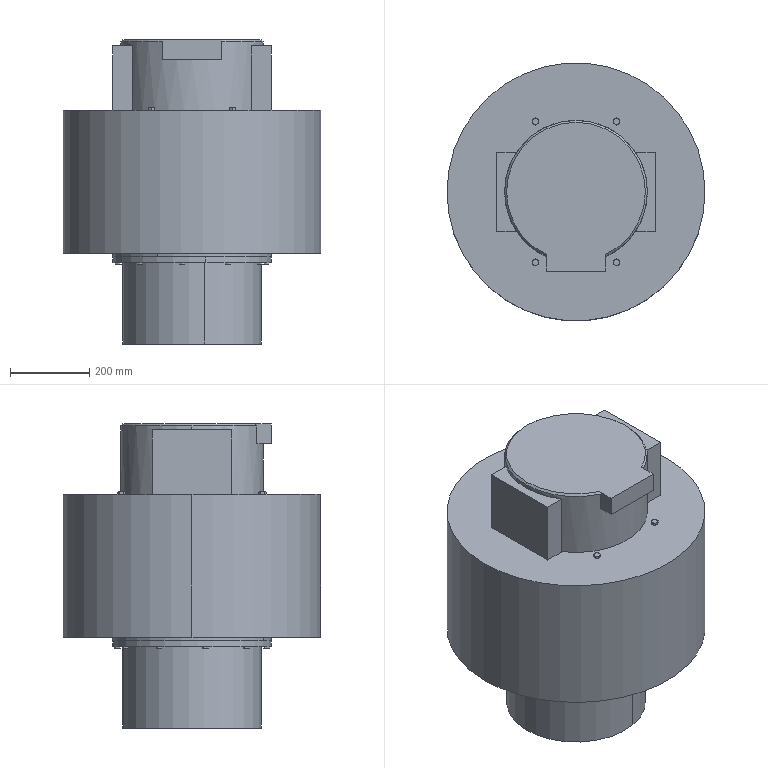Part | SolidWorks | features CompositeCurve 5 | 78 solids | 9107 faces | volume 73986218 mm3 | cylinder 3653 | sphere 2256 | torus 2025 | plane 760 | cone 405 | spline 8 | commonest cylinder face diameters 52 x450 182 x368 75.2 x294 250 x253 124.998 x195 134 x195